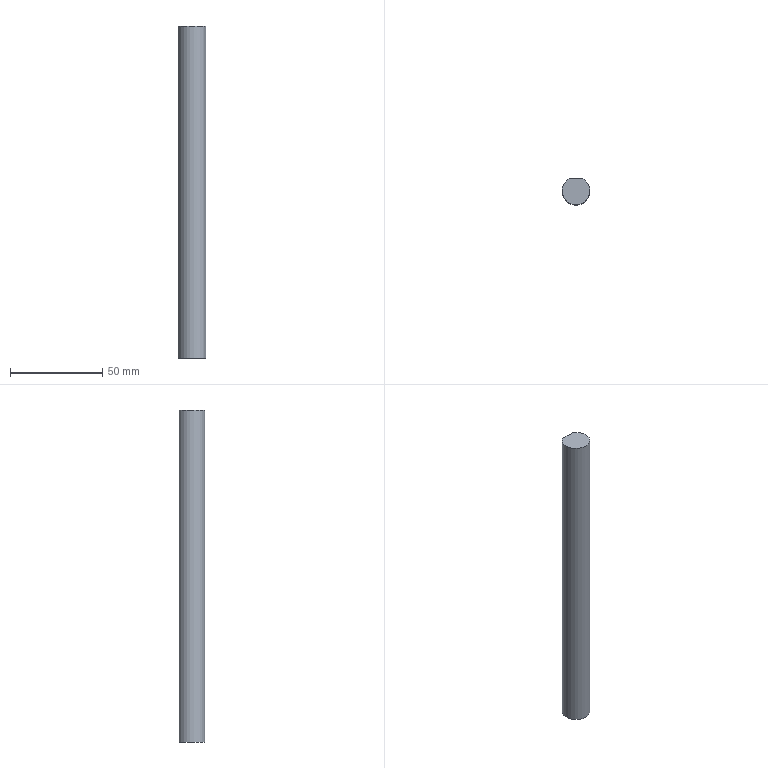NC program | NX | posted with a generic post | part box 15 x 14 x 180 mm
Whole program:
N10 G17 G21 G94 G90
(DRILLING , TOOL : ZXZ)
N12 T01 M6
N14 G54
N16 G17 G0 G90 X-80. Y0. B0. C0. S3000 M3
N18 G43 Z30. H1
N20 G94 G81 G98 Z-2. F200. R2.
N22 X-20.
N24 X40.
N26 G80
N28 G0 X40. Y0. Z30.
N30 M5
(DRILLING_COPY , TOOL : 3.3ZT)
N32 T03 M6
N34 G54
N36 G17 G0 G90 X-80. Y0. B0. C0. S2000 M3
N38 G43 Z30. H3
N40 G94 G83 G98 Z-12.091 F120. Q2. R2.
N42 X-20.
N44 X40.
N46 G80
N48 G0 X40. Y0. Z30.
N50 M5
(DRILLING_COPY_1 , TOOL : D6A45)
N52 T07 M6
N54 G54
N56 G17 G0 G90 X-80. Y0. B0. C0. S3000 M3
N58 G43 Z30. H7
N60 G94 G81 G98 Z-3. F200. R2.
N62 X-20.
N64 X40.
N66 G80
N68 G0 X40. Y0. Z30.
N70 M5
N72 M2